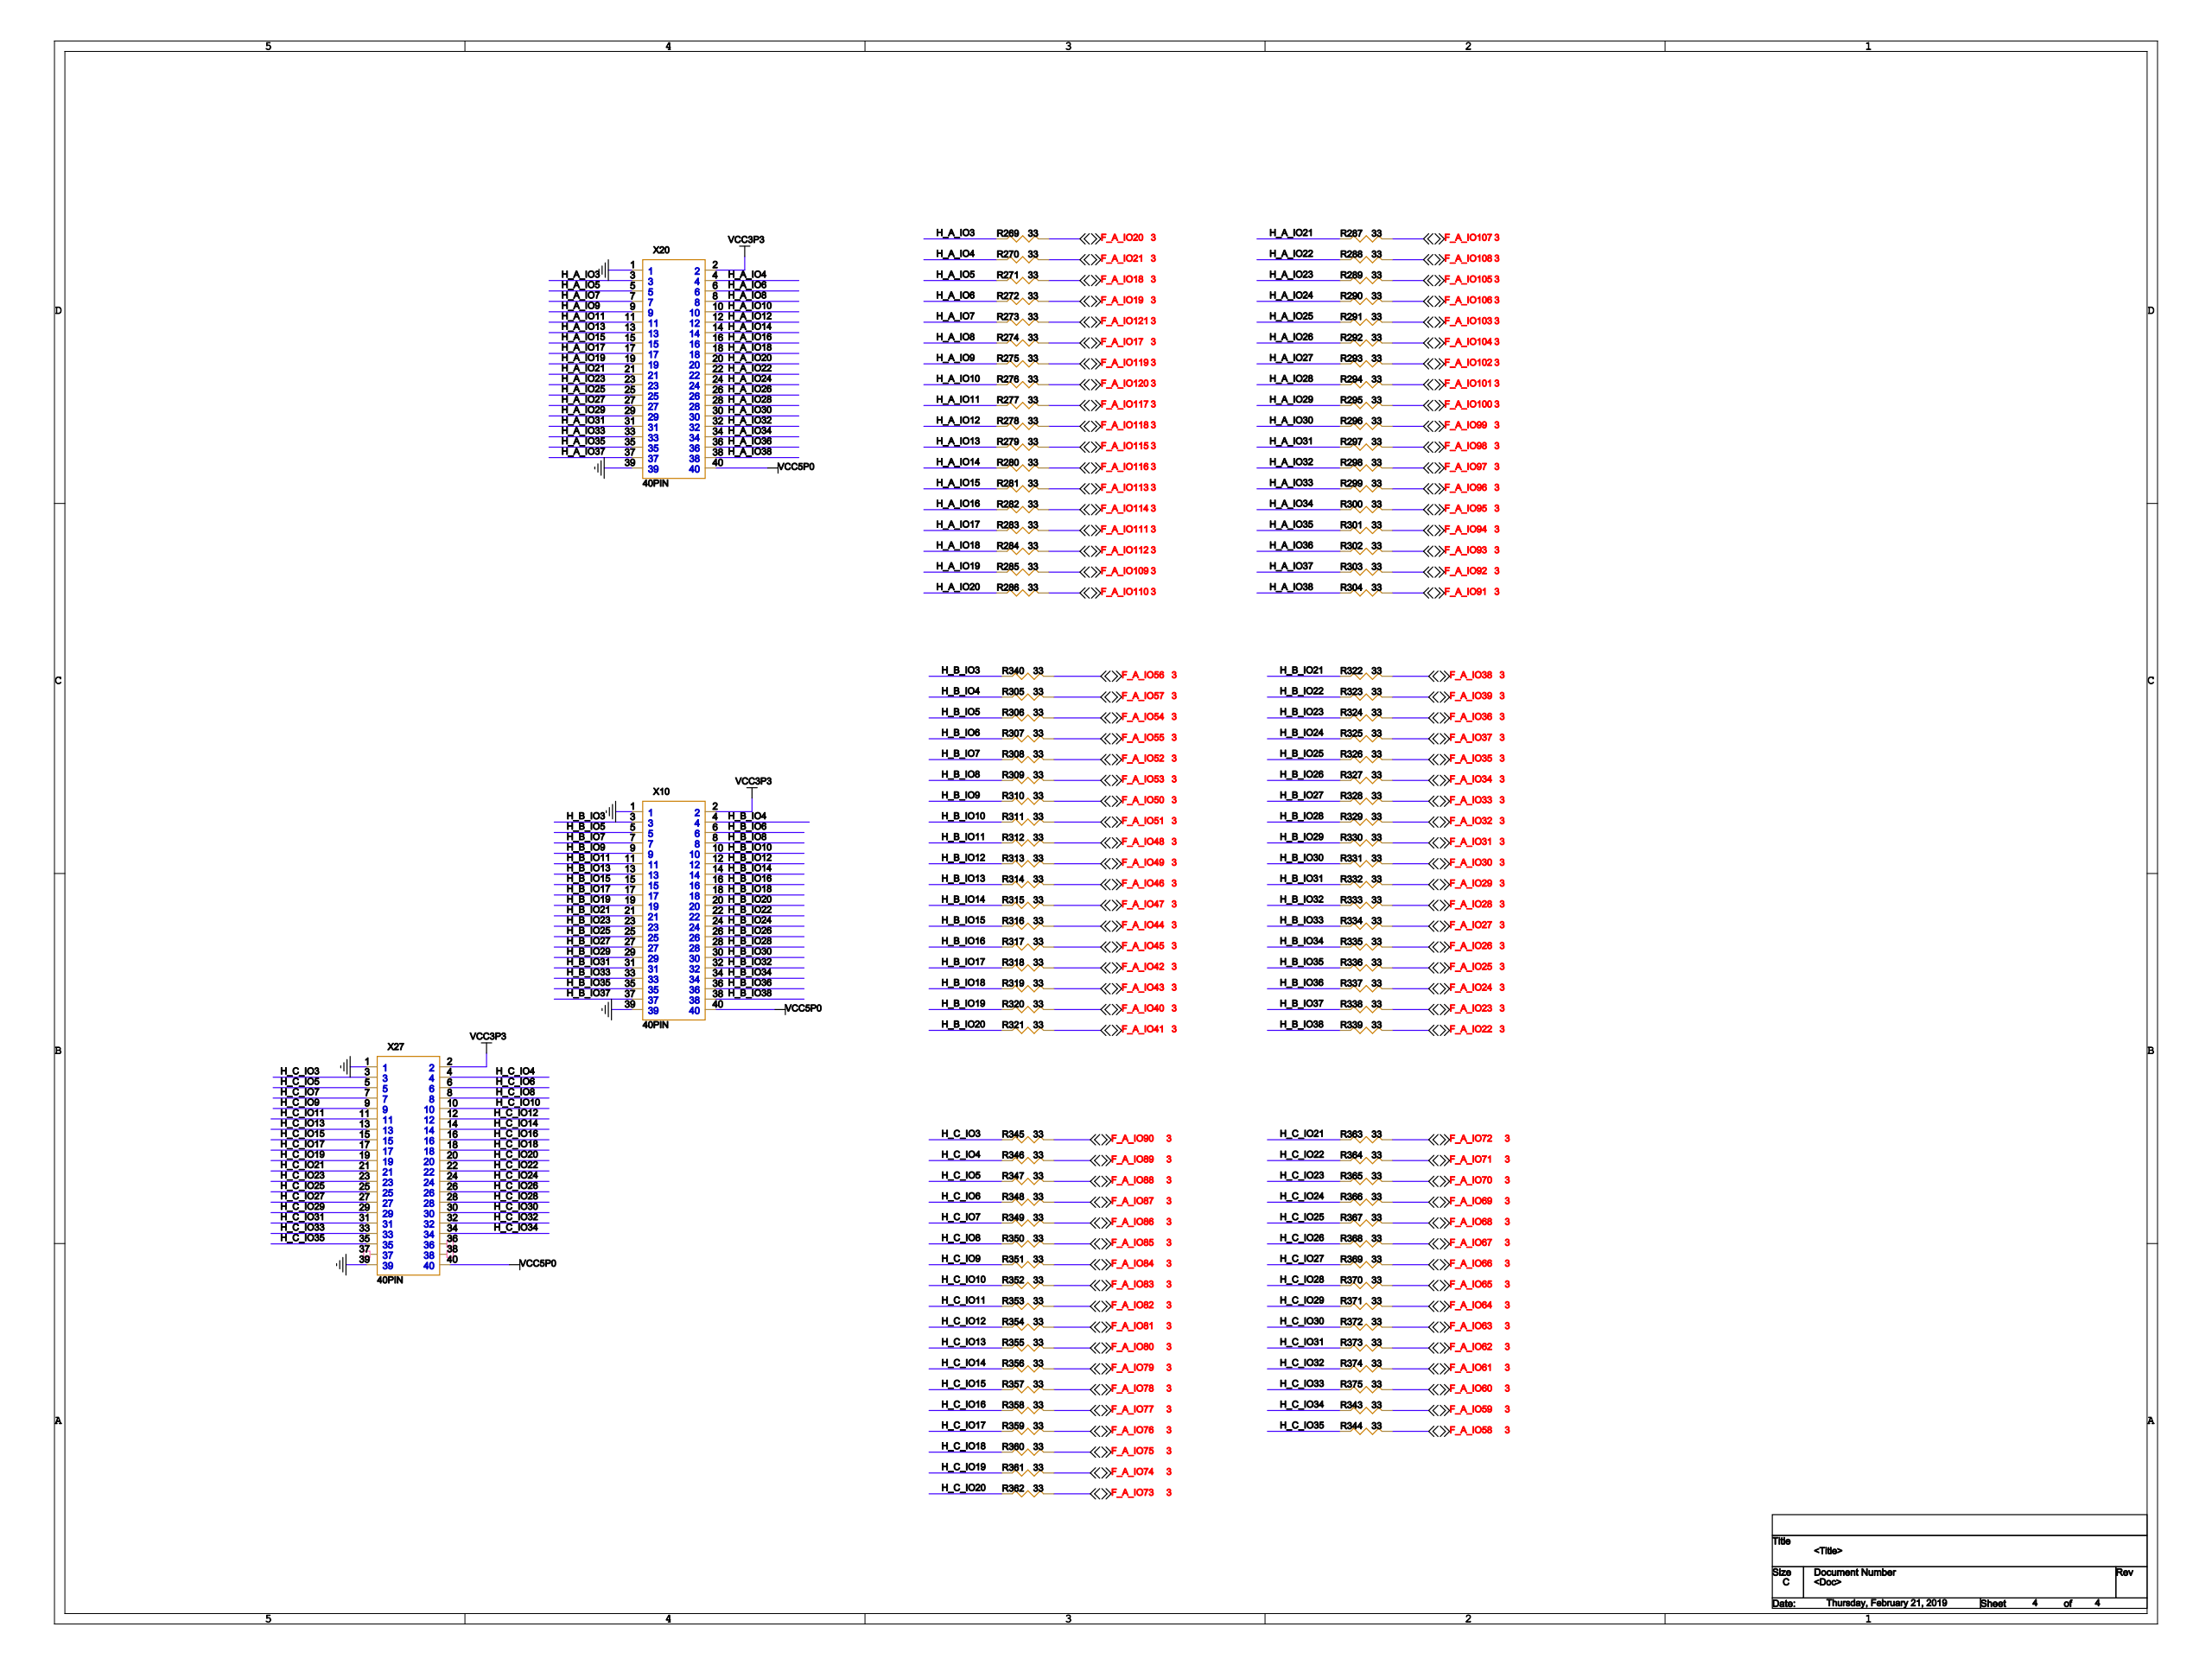Circuit board | Cadence Allegro | 174 parts | 250 nets | one sheet of the schematic
Parts on this sheet (reference | value | footprint):
R269 | 33 | R0603
R270 | 33 | R0603
R271 | 33 | R0603
R272 | 33 | R0603
R273 | 33 | R0603
R274 | 33 | R0603
R275 | 33 | R0603
R276 | 33 | R0603
R277 | 33 | R0603
R278 | 33 | R0603
R279 | 33 | R0603
R280 | 33 | R0603
R281 | 33 | R0603
R282 | 33 | R0603
R283 | 33 | R0603
R284 | 33 | R0603
R285 | 33 | R0603
R286 | 33 | R0603
R287 | 33 | R0603
R288 | 33 | R0603
R289 | 33 | R0603
R290 | 33 | R0603
R291 | 33 | R0603
R292 | 33 | R0603
R293 | 33 | R0603
R294 | 33 | R0603
R295 | 33 | R0603
R296 | 33 | R0603
R297 | 33 | R0603
R298 | 33 | R0603
R299 | 33 | R0603
R300 | 33 | R0603
R301 | 33 | R0603
R302 | 33 | R0603
R303 | 33 | R0603
R304 | 33 | R0603
R305 | 33 | R0603
R306 | 33 | R0603
R307 | 33 | R0603
R308 | 33 | R0603
R309 | 33 | R0603
R310 | 33 | R0603
R311 | 33 | R0603
R312 | 33 | R0603
R313 | 33 | R0603
R314 | 33 | R0603
R315 | 33 | R0603
R316 | 33 | R0603
R317 | 33 | R0603
R318 | 33 | R0603
R319 | 33 | R0603
R320 | 33 | R0603
R321 | 33 | R0603
R322 | 33 | R0603
R323 | 33 | R0603
R324 | 33 | R0603
R325 | 33 | R0603
R326 | 33 | R0603
R327 | 33 | R0603
R328 | 33 | R0603
R329 | 33 | R0603
R330 | 33 | R0603
R331 | 33 | R0603
R332 | 33 | R0603
R333 | 33 | R0603
R334 | 33 | R0603
R335 | 33 | R0603
R336 | 33 | R0603
R337 | 33 | R0603
R338 | 33 | R0603
R339 | 33 | R0603
R340 | 33 | R0603
R343 | 33 | R0603
R344 | 33 | R0603
R345 | 33 | R0603
R346 | 33 | R0603
R347 | 33 | R0603
R348 | 33 | R0603
R349 | 33 | R0603
R350 | 33 | R0603
R351 | 33 | R0603
R352 | 33 | R0603
R353 | 33 | R0603
R354 | 33 | R0603
R355 | 33 | R0603
R356 | 33 | R0603
R357 | 33 | R0603
R358 | 33 | R0603
R359 | 33 | R0603
R360 | 33 | R0603
R361 | 33 | R0603
R362 | 33 | R0603
R363 | 33 | R0603
R364 | 33 | R0603
R365 | 33 | R0603
R366 | 33 | R0603
R367 | 33 | R0603
R368 | 33 | R0603
R369 | 33 | R0603
R370 | 33 | R0603
R371 | 33 | R0603
R372 | 33 | R0603
R373 | 33 | R0603
R374 | 33 | R0603
R375 | 33 | R0603
X10 | 40PIN | HEADER2X20-100
X20 | 40PIN | HEADER2X20-100
X27 | 40PIN | HEADER2X20-100
Nets of these parts (net: part-pin ...):
VCC3P3: X10-2 X20-2 X27-2
VCC5P0: X10-40 X20-40 X27-40
F_A_IO38: R322-2
F_A_IO39: R323-2
F_A_IO40: R320-2
F_A_IO41: R321-2
F_A_IO42: R318-2
F_A_IO43: R319-2
F_A_IO44: R316-2
F_A_IO45: R317-2
F_A_IO46: R314-2
F_A_IO47: R315-2
F_A_IO48: R312-2
F_A_IO50: R310-2
F_A_IO51: R311-2
F_A_IO52: R308-2
F_A_IO53: R309-2
F_A_IO54: R306-2
F_A_IO55: R307-2
F_A_IO56: R340-2
F_A_IO57: R305-2
F_A_IO58: R344-2
F_A_IO59: R343-2
F_A_IO60: R375-2
F_A_IO61: R374-2
F_A_IO62: R373-2
F_A_IO63: R372-2
F_A_IO65: R370-2
F_A_IO64: R371-2
F_A_IO67: R368-2
F_A_IO66: R369-2
F_A_IO30: R331-2
F_A_IO31: R330-2
F_A_IO32: R329-2
F_A_IO34: R327-2
F_A_IO35: R326-2
F_A_IO36: R324-2
F_A_IO37: R325-2
F_A_IO21: R270-2
F_A_IO22: R339-2
F_A_IO23: R338-2
F_A_IO24: R337-2
F_A_IO25: R336-2
F_A_IO26: R335-2
F_A_IO27: R334-2
F_A_IO28: R333-2
F_A_IO29: R332-2
F_A_IO17: R274-2
F_A_IO18: R271-2
F_A_IO19: R272-2
F_A_IO20: R269-2
F_A_IO82: R353-2
F_A_IO81: R354-2
F_A_IO80: R355-2
F_A_IO79: R356-2
F_A_IO78: R357-2
F_A_IO77: R358-2
F_A_IO76: R359-2
F_A_IO75: R360-2
F_A_IO74: R361-2
F_A_IO73: R362-2
F_A_IO72: R363-2
F_A_IO71: R364-2
F_A_IO70: R365-2
F_A_IO69: R366-2
F_A_IO68: R367-2
F_A_IO90: R345-2
F_A_IO89: R346-2
F_A_IO88: R347-2
F_A_IO87: R348-2
F_A_IO86: R349-2
F_A_IO85: R350-2
F_A_IO84: R351-2
F_A_IO83: R352-2
F_A_IO113: R281-2
F_A_IO112: R284-2
F_A_IO111: R283-2
F_A_IO110: R286-2
F_A_IO109: R285-2
F_A_IO108: R288-2
F_A_IO107: R287-2
F_A_IO106: R290-2
F_A_IO105: R289-2
F_A_IO104: R292-2
F_A_IO103: R291-2
F_A_IO102: R293-2
F_A_IO101: R294-2
F_A_IO100: R295-2
F_A_IO99: R296-2
F_A_IO98: R297-2
F_A_IO97: R298-2
F_A_IO96: R299-2
F_A_IO95: R300-2
F_A_IO94: R301-2
F_A_IO93: R302-2
F_A_IO92: R303-2
F_A_IO91: R304-2
F_A_IO121: R273-2
F_A_IO120: R276-2
F_A_IO119: R275-2
F_A_IO118: R278-2
F_A_IO117: R277-2
F_A_IO116: R280-2
F_A_IO115: R279-2
F_A_IO114: R282-2
F_A_IO49: R313-2
F_A_IO33: R328-2
H_C_IO30: R372-1 X27-30
H_C_IO31: R373-1 X27-31
H_C_IO32: R374-1 X27-32
H_C_IO33: R375-1 X27-33
H_A_IO3: R269-1 X20-3
H_A_IO4: R270-1 X20-4
H_A_IO5: R271-1 X20-5
H_A_IO6: R272-1 X20-6
H_A_IO7: R273-1 X20-7
H_A_IO8: R274-1 X20-8
H_A_IO9: R275-1 X20-9
H_A_IO10: R276-1 X20-10
H_A_IO11: R277-1 X20-11
H_A_IO12: R278-1 X20-12
H_A_IO13: R279-1 X20-13
H_A_IO14: R280-1 X20-14
H_A_IO15: R281-1 X20-15
H_A_IO16: R282-1 X20-16
H_A_IO17: R283-1 X20-17
H_A_IO18: R284-1 X20-18
H_A_IO19: R285-1 X20-19
H_A_IO20: R286-1 X20-20
H_A_IO21: R287-1 X20-21
H_A_IO22: R288-1 X20-22
H_A_IO23: R289-1 X20-23
H_A_IO24: R290-1 X20-24
H_A_IO25: R291-1 X20-25
H_A_IO26: R292-1 X20-26
H_A_IO27: R293-1 X20-27
H_A_IO28: R294-1 X20-28
H_A_IO29: R295-1 X20-29
H_A_IO30: R296-1 X20-30
H_A_IO31: R297-1 X20-31
H_A_IO32: R298-1 X20-32
H_A_IO33: R299-1 X20-33
H_A_IO34: R300-1 X20-34
H_A_IO35: R301-1 X20-35
H_A_IO36: R302-1 X20-36
H_A_IO37: R303-1 X20-37
H_A_IO38: R304-1 X20-38
H_B_IO4: R305-1 X10-4
H_B_IO5: R306-1 X10-5
H_B_IO6: R307-1 X10-6
H_B_IO7: R308-1 X10-7
H_B_IO8: R309-1 X10-8
H_B_IO9: R310-1 X10-9
H_B_IO10: R311-1 X10-10
H_B_IO11: R312-1 X10-11
H_B_IO12: R313-1 X10-12
H_B_IO13: R314-1 X10-13
H_B_IO14: R315-1 X10-14
H_B_IO15: R316-1 X10-15
H_B_IO16: R317-1 X10-16
H_B_IO17: R318-1 X10-17
H_B_IO18: R319-1 X10-18
H_B_IO19: R320-1 X10-19
H_B_IO20: R321-1 X10-20
H_B_IO21: R322-1 X10-21
H_B_IO22: R323-1 X10-22
H_B_IO23: R324-1 X10-23
H_B_IO24: R325-1 X10-24
H_B_IO25: R326-1 X10-25
H_B_IO26: R327-1 X10-26
H_B_IO27: R328-1 X10-27
H_B_IO28: R329-1 X10-28
H_B_IO29: R330-1 X10-29
H_B_IO30: R331-1 X10-30
H_B_IO31: R332-1 X10-31
H_B_IO32: R333-1 X10-32
H_B_IO33: R334-1 X10-33
H_B_IO34: R335-1 X10-34
H_B_IO35: R336-1 X10-35
H_B_IO36: R337-1 X10-36
H_B_IO37: R338-1 X10-37
H_B_IO38: R339-1 X10-38
H_B_IO3: R340-1 X10-3
H_C_IO34: R343-1 X27-34
H_C_IO35: R344-1 X27-35
H_C_IO3: R345-1 X27-3
H_C_IO4: R346-1 X27-4
H_C_IO5: R347-1 X27-5
H_C_IO6: R348-1 X27-6
H_C_IO7: R349-1 X27-7
H_C_IO8: R350-1 X27-8
H_C_IO9: R351-1 X27-9
H_C_IO10: R352-1 X27-10
H_C_IO11: R353-1 X27-11
H_C_IO12: R354-1 X27-12
H_C_IO13: R355-1 X27-13
H_C_IO14: R356-1 X27-14
H_C_IO15: R357-1 X27-15
H_C_IO16: R358-1 X27-16
H_C_IO17: R359-1 X27-17
H_C_IO18: R360-1 X27-18
H_C_IO19: R361-1 X27-19
H_C_IO20: R362-1 X27-20
H_C_IO21: R363-1 X27-21
H_C_IO22: R364-1 X27-22
H_C_IO23: R365-1 X27-23
H_C_IO24: R366-1 X27-24
H_C_IO25: R367-1 X27-25
H_C_IO26: R368-1 X27-26
H_C_IO27: R369-1 X27-27
H_C_IO28: R370-1 X27-28
H_C_IO29: R371-1 X27-29